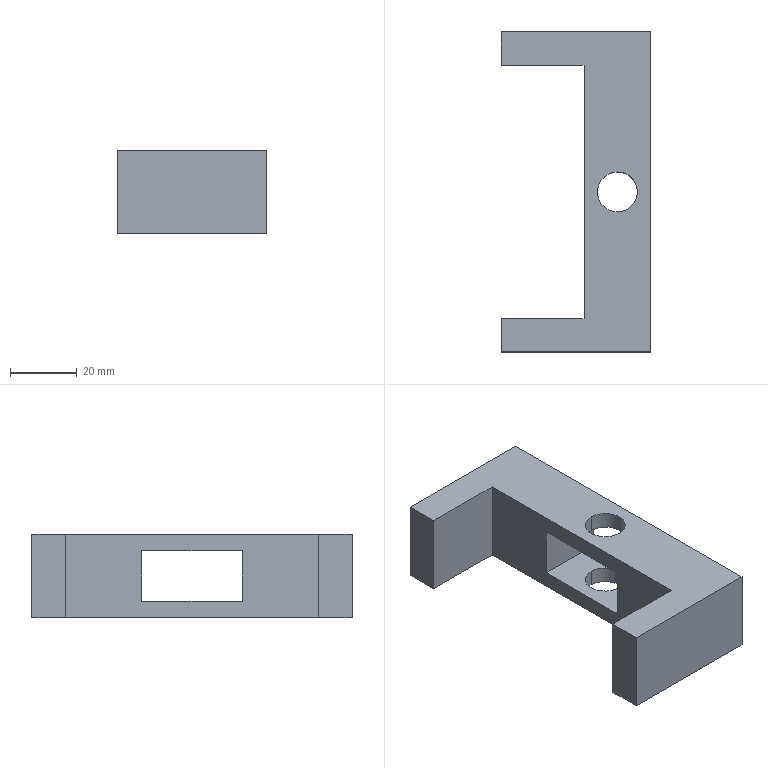Part | STEP file | Positioning_id1954_x_t | 1 solid | 18 faces | box 44.8 x 96 x 25 mm | volume 50269 mm3 | plane 14 | cylinder 4 | commonest cylinder face diameters 12 x4